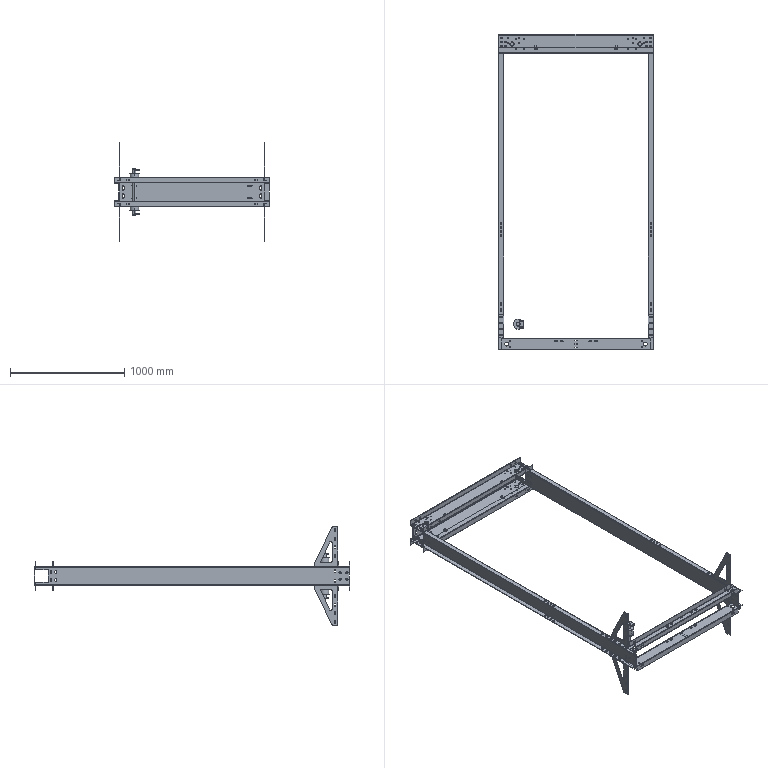Part | SolidWorks | features ReferencePattern 10, MirrorCompFeat 7, LocalLPattern 1 | 15 solids | 1292 faces | box 1350 x 2756 x 860 mm | volume 17468033 mm3 | cylinder 756 | plane 528 | torus 4 | cone 4 | commonest cylinder face diameters 13 x232 14 x156 12 x54 11 x52 6 x48 8.5 x48